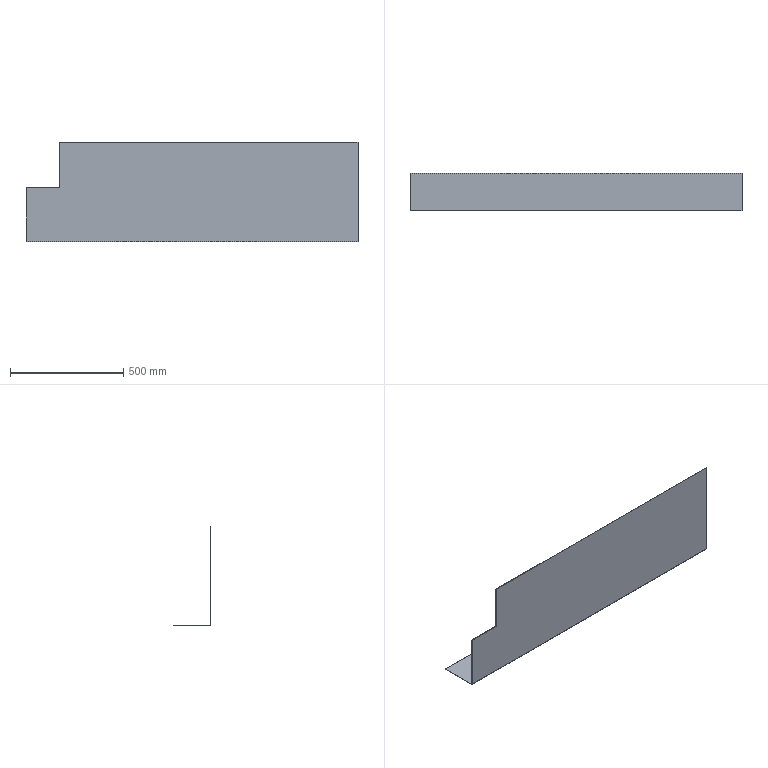Part | 1 solid | 16 faces | box 1465 x 167 x 440 mm | volume 1027988 mm3 | plane 14 | cylinder 2 | commonest cylinder face diameters 1.473 x1 3.873 x1
STEP:
#1=CARTESIAN_POINT('',(732.5,-81.563,0.));
#2=VERTEX_POINT('',#1);
#3=CARTESIAN_POINT('',(732.5,83.5,0.));
#4=VERTEX_POINT('',#3);
#5=CARTESIAN_POINT('',(732.5,83.5,0.));
#6=DIRECTION('',(0.,1.,0.));
#7=VECTOR('',#6,1000.);
#8=LINE('',#5,#7);
#9=EDGE_CURVE('',#2,#4,#8,.T.);
#10=ORIENTED_EDGE('',*,*,#9,.F.);
#11=CARTESIAN_POINT('',(732.5,-81.563,-1.2));
#12=VERTEX_POINT('',#11);
#13=CARTESIAN_POINT('',(732.5,-81.563,0.));
#14=DIRECTION('',(0.,0.,-1.));
#15=VECTOR('',#14,1000.);
#16=LINE('',#13,#15);
#17=EDGE_CURVE('',#2,#12,#16,.T.);
#18=ORIENTED_EDGE('',*,*,#17,.T.);
#19=CARTESIAN_POINT('',(732.5,83.5,-1.2));
#20=VERTEX_POINT('',#19);
#21=CARTESIAN_POINT('',(732.5,83.5,-1.2));
#22=DIRECTION('',(0.,1.,0.));
#23=VECTOR('',#22,1000.);
#24=LINE('',#21,#23);
#25=EDGE_CURVE('',#12,#20,#24,.T.);
#26=ORIENTED_EDGE('',*,*,#25,.T.);
#27=CARTESIAN_POINT('',(732.5,83.5,-1.2));
#28=DIRECTION('',(0.,0.,1.));
#29=VECTOR('',#28,1000.);
#30=LINE('',#27,#29);
#31=EDGE_CURVE('',#20,#4,#30,.T.);
#32=ORIENTED_EDGE('',*,*,#31,.T.);
#33=EDGE_LOOP('',(#10,#18,#26,#32));
#34=FACE_OUTER_BOUND('',#33,.T.);
#35=CARTESIAN_POINT('',(732.5,83.5,-1.2));
#36=DIRECTION('',(1.,0.,0.));
#37=DIRECTION('',(0.,1.,0.));
#38=AXIS2_PLACEMENT_3D('',#35,#36,#37);
#39=PLANE('',#38);
#40=ADVANCED_FACE('',(#34),#39,.T.);
#41=CARTESIAN_POINT('',(-732.5,-81.563,-1.2));
#42=VERTEX_POINT('',#41);
#43=CARTESIAN_POINT('',(732.5,-81.563,-1.2));
#44=DIRECTION('',(-1.,0.,0.));
#45=VECTOR('',#44,1000.);
#46=LINE('',#43,#45);
#47=EDGE_CURVE('',#12,#42,#46,.T.);
#48=ORIENTED_EDGE('',*,*,#47,.T.);
#49=CARTESIAN_POINT('',(-732.5,83.5,-1.2));
#50=VERTEX_POINT('',#49);
#51=CARTESIAN_POINT('',(-732.5,83.5,-1.2));
#52=DIRECTION('',(0.,-1.,0.));
#53=VECTOR('',#52,1000.);
#54=LINE('',#51,#53);
#55=EDGE_CURVE('',#50,#42,#54,.T.);
#56=ORIENTED_EDGE('',*,*,#55,.F.);
#57=CARTESIAN_POINT('',(-732.5,83.5,-1.2));
#58=DIRECTION('',(-1.,0.,0.));
#59=VECTOR('',#58,1000.);
#60=LINE('',#57,#59);
#61=EDGE_CURVE('',#20,#50,#60,.T.);
#62=ORIENTED_EDGE('',*,*,#61,.F.);
#63=ORIENTED_EDGE('',*,*,#25,.F.);
#64=EDGE_LOOP('',(#48,#56,#62,#63));
#65=FACE_OUTER_BOUND('',#64,.T.);
#66=CARTESIAN_POINT('',(0.,0.,-1.2));
#67=DIRECTION('',(0.,0.,1.));
#68=DIRECTION('',(1.,0.,0.));
#69=AXIS2_PLACEMENT_3D('',#66,#67,#68);
#70=PLANE('',#69);
#71=ADVANCED_FACE('',(#65),#70,.F.);
#72=CARTESIAN_POINT('',(-732.5,83.5,0.));
#73=VERTEX_POINT('',#72);
#74=CARTESIAN_POINT('',(-732.5,-81.563,0.));
#75=VERTEX_POINT('',#74);
#76=CARTESIAN_POINT('',(-732.5,83.5,0.));
#77=DIRECTION('',(0.,-1.,0.));
#78=VECTOR('',#77,1000.);
#79=LINE('',#76,#78);
#80=EDGE_CURVE('',#73,#75,#79,.T.);
#81=ORIENTED_EDGE('',*,*,#80,.T.);
#82=CARTESIAN_POINT('',(732.5,-81.563,0.));
#83=DIRECTION('',(-1.,0.,0.));
#84=VECTOR('',#83,1000.);
#85=LINE('',#82,#84);
#86=EDGE_CURVE('',#2,#75,#85,.T.);
#87=ORIENTED_EDGE('',*,*,#86,.F.);
#88=ORIENTED_EDGE('',*,*,#9,.T.);
#89=CARTESIAN_POINT('',(-732.5,83.5,0.));
#90=DIRECTION('',(-1.,0.,0.));
#91=VECTOR('',#90,1000.);
#92=LINE('',#89,#91);
#93=EDGE_CURVE('',#4,#73,#92,.T.);
#94=ORIENTED_EDGE('',*,*,#93,.T.);
#95=EDGE_LOOP('',(#81,#87,#88,#94));
#96=FACE_OUTER_BOUND('',#95,.T.);
#97=CARTESIAN_POINT('',(0.,0.,0.));
#98=DIRECTION('',(0.,0.,1.));
#99=DIRECTION('',(1.,0.,0.));
#100=AXIS2_PLACEMENT_3D('',#97,#98,#99);
#101=PLANE('',#100);
#102=ADVANCED_FACE('',(#96),#101,.T.);
#103=CARTESIAN_POINT('',(-732.5,-81.563,0.));
#104=DIRECTION('',(0.,0.,-1.));
#105=VECTOR('',#104,1000.);
#106=LINE('',#103,#105);
#107=EDGE_CURVE('',#75,#42,#106,.T.);
#108=ORIENTED_EDGE('',*,*,#107,.F.);
#109=ORIENTED_EDGE('',*,*,#80,.F.);
#110=CARTESIAN_POINT('',(-732.5,83.5,-1.2));
#111=DIRECTION('',(0.,0.,1.));
#112=VECTOR('',#111,1000.);
#113=LINE('',#110,#112);
#114=EDGE_CURVE('',#50,#73,#113,.T.);
#115=ORIENTED_EDGE('',*,*,#114,.F.);
#116=ORIENTED_EDGE('',*,*,#55,.T.);
#117=EDGE_LOOP('',(#108,#109,#115,#116));
#118=FACE_OUTER_BOUND('',#117,.T.);
#119=CARTESIAN_POINT('',(-732.5,83.5,-1.2));
#120=DIRECTION('',(-1.,0.,0.));
#121=DIRECTION('',(0.,0.,1.));
#122=AXIS2_PLACEMENT_3D('',#119,#120,#121);
#123=PLANE('',#122);
#124=ADVANCED_FACE('',(#118),#123,.T.);
#125=ORIENTED_EDGE('',*,*,#93,.F.);
#126=ORIENTED_EDGE('',*,*,#31,.F.);
#127=ORIENTED_EDGE('',*,*,#61,.T.);
#128=ORIENTED_EDGE('',*,*,#114,.T.);
#129=EDGE_LOOP('',(#125,#126,#127,#128));
#130=FACE_OUTER_BOUND('',#129,.T.);
#131=CARTESIAN_POINT('',(-732.5,83.5,-1.2));
#132=DIRECTION('',(0.,1.,0.));
#133=DIRECTION('',(0.,0.,1.));
#134=AXIS2_PLACEMENT_3D('',#131,#132,#133);
#135=PLANE('',#134);
#136=ADVANCED_FACE('',(#130),#135,.T.);
#137=CARTESIAN_POINT('',(-732.5,-82.3,0.7366));
#138=VERTEX_POINT('',#137);
#139=CARTESIAN_POINT('',(-732.5,-83.5,0.7366));
#140=VERTEX_POINT('',#139);
#141=CARTESIAN_POINT('',(-732.5,-83.5,0.7366));
#142=DIRECTION('',(0.,-1.,0.));
#143=VECTOR('',#142,1000.);
#144=LINE('',#141,#143);
#145=EDGE_CURVE('',#138,#140,#144,.T.);
#146=ORIENTED_EDGE('',*,*,#145,.F.);
#147=CARTESIAN_POINT('',(-732.5,-81.563,0.7366));
#148=DIRECTION('',(-1.,0.,0.));
#149=DIRECTION('',(0.,0.,-1.));
#150=AXIS2_PLACEMENT_3D('',#147,#148,#149);
#151=CIRCLE('',#150,0.7366);
#152=EDGE_CURVE('',#75,#138,#151,.T.);
#153=ORIENTED_EDGE('',*,*,#152,.F.);
#154=ORIENTED_EDGE('',*,*,#107,.T.);
#155=CARTESIAN_POINT('',(-732.5,-81.563,0.7366));
#156=DIRECTION('',(-1.,0.,0.));
#157=DIRECTION('',(0.,0.,-1.));
#158=AXIS2_PLACEMENT_3D('',#155,#156,#157);
#159=CIRCLE('',#158,1.937);
#160=EDGE_CURVE('',#42,#140,#159,.T.);
#161=ORIENTED_EDGE('',*,*,#160,.T.);
#162=EDGE_LOOP('',(#146,#153,#154,#161));
#163=FACE_OUTER_BOUND('',#162,.T.);
#164=CARTESIAN_POINT('',(-732.5,-81.563,0.7366));
#165=DIRECTION('',(-1.,0.,0.));
#166=DIRECTION('',(0.,0.,1.));
#167=AXIS2_PLACEMENT_3D('',#164,#165,#166);
#168=PLANE('',#167);
#169=ADVANCED_FACE('',(#163),#168,.T.);
#170=CARTESIAN_POINT('',(732.5,-82.3,0.7366));
#171=VERTEX_POINT('',#170);
#172=CARTESIAN_POINT('',(732.5,-81.563,0.7366));
#173=DIRECTION('',(1.,0.,0.));
#174=DIRECTION('',(0.,0.,-1.));
#175=AXIS2_PLACEMENT_3D('',#172,#173,#174);
#176=CIRCLE('',#175,0.7366);
#177=EDGE_CURVE('',#171,#2,#176,.T.);
#178=ORIENTED_EDGE('',*,*,#177,.F.);
#179=CARTESIAN_POINT('',(732.5,-83.5,0.7366));
#180=VERTEX_POINT('',#179);
#181=CARTESIAN_POINT('',(732.5,-82.3,0.7366));
#182=DIRECTION('',(0.,-1.,0.));
#183=VECTOR('',#182,1000.);
#184=LINE('',#181,#183);
#185=EDGE_CURVE('',#171,#180,#184,.T.);
#186=ORIENTED_EDGE('',*,*,#185,.T.);
#187=CARTESIAN_POINT('',(732.5,-81.563,0.7366));
#188=DIRECTION('',(1.,0.,0.));
#189=DIRECTION('',(0.,0.,-1.));
#190=AXIS2_PLACEMENT_3D('',#187,#188,#189);
#191=CIRCLE('',#190,1.937);
#192=EDGE_CURVE('',#180,#12,#191,.T.);
#193=ORIENTED_EDGE('',*,*,#192,.T.);
#194=ORIENTED_EDGE('',*,*,#17,.F.);
#195=EDGE_LOOP('',(#178,#186,#193,#194));
#196=FACE_OUTER_BOUND('',#195,.T.);
#197=CARTESIAN_POINT('',(732.5,-81.563,0.7366));
#198=DIRECTION('',(-1.,0.,0.));
#199=DIRECTION('',(0.,0.,1.));
#200=AXIS2_PLACEMENT_3D('',#197,#198,#199);
#201=PLANE('',#200);
#202=ADVANCED_FACE('',(#196),#201,.F.);
#203=ORIENTED_EDGE('',*,*,#47,.F.);
#204=ORIENTED_EDGE('',*,*,#192,.F.);
#205=CARTESIAN_POINT('',(0.,-83.5,0.7366));
#206=DIRECTION('',(1.,0.,0.));
#207=VECTOR('',#206,1000.);
#208=LINE('',#205,#207);
#209=EDGE_CURVE('',#140,#180,#208,.T.);
#210=ORIENTED_EDGE('',*,*,#209,.F.);
#211=ORIENTED_EDGE('',*,*,#160,.F.);
#212=EDGE_LOOP('',(#203,#204,#210,#211));
#213=FACE_OUTER_BOUND('',#212,.T.);
#214=CARTESIAN_POINT('',(732.5,-81.563,0.7366));
#215=DIRECTION('',(1.,0.,0.));
#216=DIRECTION('',(0.,-1.,0.));
#217=AXIS2_PLACEMENT_3D('',#214,#215,#216);
#218=CYLINDRICAL_SURFACE('',#217,1.937);
#219=ADVANCED_FACE('',(#213),#218,.T.);
#220=ORIENTED_EDGE('',*,*,#86,.T.);
#221=ORIENTED_EDGE('',*,*,#152,.T.);
#222=CARTESIAN_POINT('',(-732.5,-82.3,0.7366));
#223=DIRECTION('',(1.,0.,0.));
#224=VECTOR('',#223,1000.);
#225=LINE('',#222,#224);
#226=EDGE_CURVE('',#138,#171,#225,.T.);
#227=ORIENTED_EDGE('',*,*,#226,.T.);
#228=ORIENTED_EDGE('',*,*,#177,.T.);
#229=EDGE_LOOP('',(#220,#221,#227,#228));
#230=FACE_OUTER_BOUND('',#229,.T.);
#231=CARTESIAN_POINT('',(732.5,-81.563,0.7366));
#232=DIRECTION('',(1.,0.,0.));
#233=DIRECTION('',(0.,-1.,0.));
#234=AXIS2_PLACEMENT_3D('',#231,#232,#233);
#235=CYLINDRICAL_SURFACE('',#234,0.7366);
#236=ADVANCED_FACE('',(#230),#235,.F.);
#237=CARTESIAN_POINT('',(732.5,-83.5,438.8));
#238=VERTEX_POINT('',#237);
#239=CARTESIAN_POINT('',(732.5,-83.5,0.));
#240=DIRECTION('',(0.,0.,-1.));
#241=VECTOR('',#240,1000.);
#242=LINE('',#239,#241);
#243=EDGE_CURVE('',#238,#180,#242,.T.);
#244=ORIENTED_EDGE('',*,*,#243,.T.);
#245=ORIENTED_EDGE('',*,*,#185,.F.);
#246=CARTESIAN_POINT('',(732.5,-82.3,438.8));
#247=VERTEX_POINT('',#246);
#248=CARTESIAN_POINT('',(732.5,-82.3,0.));
#249=DIRECTION('',(0.,0.,-1.));
#250=VECTOR('',#249,1000.);
#251=LINE('',#248,#250);
#252=EDGE_CURVE('',#247,#171,#251,.T.);
#253=ORIENTED_EDGE('',*,*,#252,.F.);
#254=CARTESIAN_POINT('',(732.5,-83.5,438.8));
#255=DIRECTION('',(0.,1.,0.));
#256=VECTOR('',#255,1000.);
#257=LINE('',#254,#256);
#258=EDGE_CURVE('',#238,#247,#257,.T.);
#259=ORIENTED_EDGE('',*,*,#258,.F.);
#260=EDGE_LOOP('',(#244,#245,#253,#259));
#261=FACE_OUTER_BOUND('',#260,.T.);
#262=CARTESIAN_POINT('',(732.5,-83.5,0.));
#263=DIRECTION('',(1.,0.,0.));
#264=DIRECTION('',(0.,0.,-1.));
#265=AXIS2_PLACEMENT_3D('',#262,#263,#264);
#266=PLANE('',#265);
#267=ADVANCED_FACE('',(#261),#266,.T.);
#268=CARTESIAN_POINT('',(-732.5,-83.5,238.8));
#269=VERTEX_POINT('',#268);
#270=CARTESIAN_POINT('',(-732.5,-82.3,238.8));
#271=VERTEX_POINT('',#270);
#272=CARTESIAN_POINT('',(-732.5,-83.5,238.8));
#273=DIRECTION('',(0.,1.,0.));
#274=VECTOR('',#273,1000.);
#275=LINE('',#272,#274);
#276=EDGE_CURVE('',#269,#271,#275,.T.);
#277=ORIENTED_EDGE('',*,*,#276,.T.);
#278=CARTESIAN_POINT('',(-732.5,-82.3,0.));
#279=DIRECTION('',(0.,0.,1.));
#280=VECTOR('',#279,1000.);
#281=LINE('',#278,#280);
#282=EDGE_CURVE('',#138,#271,#281,.T.);
#283=ORIENTED_EDGE('',*,*,#282,.F.);
#284=ORIENTED_EDGE('',*,*,#145,.T.);
#285=CARTESIAN_POINT('',(-732.5,-83.5,438.8));
#286=DIRECTION('',(0.,0.,1.));
#287=VECTOR('',#286,1000.);
#288=LINE('',#285,#287);
#289=EDGE_CURVE('',#140,#269,#288,.T.);
#290=ORIENTED_EDGE('',*,*,#289,.T.);
#291=EDGE_LOOP('',(#277,#283,#284,#290));
#292=FACE_OUTER_BOUND('',#291,.T.);
#293=CARTESIAN_POINT('',(-732.5,-83.5,438.8));
#294=DIRECTION('',(-1.,0.,0.));
#295=DIRECTION('',(0.,0.,1.));
#296=AXIS2_PLACEMENT_3D('',#293,#294,#295);
#297=PLANE('',#296);
#298=ADVANCED_FACE('',(#292),#297,.T.);
#299=CARTESIAN_POINT('',(-582.5,-83.5,238.8));
#300=VERTEX_POINT('',#299);
#301=CARTESIAN_POINT('',(-732.5,-83.5,238.8));
#302=DIRECTION('',(-1.,0.,0.));
#303=VECTOR('',#302,1000.);
#304=LINE('',#301,#303);
#305=EDGE_CURVE('',#300,#269,#304,.T.);
#306=ORIENTED_EDGE('',*,*,#305,.T.);
#307=ORIENTED_EDGE('',*,*,#289,.F.);
#308=ORIENTED_EDGE('',*,*,#209,.T.);
#309=ORIENTED_EDGE('',*,*,#243,.F.);
#310=CARTESIAN_POINT('',(-582.5,-83.5,438.8));
#311=VERTEX_POINT('',#310);
#312=CARTESIAN_POINT('',(732.5,-83.5,438.8));
#313=DIRECTION('',(1.,0.,0.));
#314=VECTOR('',#313,1000.);
#315=LINE('',#312,#314);
#316=EDGE_CURVE('',#311,#238,#315,.T.);
#317=ORIENTED_EDGE('',*,*,#316,.F.);
#318=CARTESIAN_POINT('',(-582.5,-83.5,438.8));
#319=DIRECTION('',(0.,0.,-1.));
#320=VECTOR('',#319,1000.);
#321=LINE('',#318,#320);
#322=EDGE_CURVE('',#311,#300,#321,.T.);
#323=ORIENTED_EDGE('',*,*,#322,.T.);
#324=EDGE_LOOP('',(#306,#307,#308,#309,#317,#323));
#325=FACE_OUTER_BOUND('',#324,.T.);
#326=CARTESIAN_POINT('',(0.,-83.5,0.));
#327=DIRECTION('',(0.,-1.,0.));
#328=DIRECTION('',(0.,0.,-1.));
#329=AXIS2_PLACEMENT_3D('',#326,#327,#328);
#330=PLANE('',#329);
#331=ADVANCED_FACE('',(#325),#330,.T.);
#332=ORIENTED_EDGE('',*,*,#282,.T.);
#333=CARTESIAN_POINT('',(-582.5,-82.3,238.8));
#334=VERTEX_POINT('',#333);
#335=CARTESIAN_POINT('',(-732.5,-82.3,238.8));
#336=DIRECTION('',(-1.,0.,0.));
#337=VECTOR('',#336,1000.);
#338=LINE('',#335,#337);
#339=EDGE_CURVE('',#334,#271,#338,.T.);
#340=ORIENTED_EDGE('',*,*,#339,.F.);
#341=CARTESIAN_POINT('',(-582.5,-82.3,438.8));
#342=VERTEX_POINT('',#341);
#343=CARTESIAN_POINT('',(-582.5,-82.3,438.8));
#344=DIRECTION('',(0.,0.,-1.));
#345=VECTOR('',#344,1000.);
#346=LINE('',#343,#345);
#347=EDGE_CURVE('',#342,#334,#346,.T.);
#348=ORIENTED_EDGE('',*,*,#347,.F.);
#349=CARTESIAN_POINT('',(0.,-82.3,438.8));
#350=DIRECTION('',(1.,0.,0.));
#351=VECTOR('',#350,1000.);
#352=LINE('',#349,#351);
#353=EDGE_CURVE('',#342,#247,#352,.T.);
#354=ORIENTED_EDGE('',*,*,#353,.T.);
#355=ORIENTED_EDGE('',*,*,#252,.T.);
#356=ORIENTED_EDGE('',*,*,#226,.F.);
#357=EDGE_LOOP('',(#332,#340,#348,#354,#355,#356));
#358=FACE_OUTER_BOUND('',#357,.T.);
#359=CARTESIAN_POINT('',(0.,-82.3,0.));
#360=DIRECTION('',(0.,-1.,0.));
#361=DIRECTION('',(0.,0.,-1.));
#362=AXIS2_PLACEMENT_3D('',#359,#360,#361);
#363=PLANE('',#362);
#364=ADVANCED_FACE('',(#358),#363,.F.);
#365=CARTESIAN_POINT('',(-582.5,-83.5,438.8));
#366=DIRECTION('',(0.,1.,0.));
#367=VECTOR('',#366,1000.);
#368=LINE('',#365,#367);
#369=EDGE_CURVE('',#311,#342,#368,.T.);
#370=ORIENTED_EDGE('',*,*,#369,.F.);
#371=ORIENTED_EDGE('',*,*,#316,.T.);
#372=ORIENTED_EDGE('',*,*,#258,.T.);
#373=ORIENTED_EDGE('',*,*,#353,.F.);
#374=EDGE_LOOP('',(#370,#371,#372,#373));
#375=FACE_OUTER_BOUND('',#374,.T.);
#376=CARTESIAN_POINT('',(732.5,-83.5,438.8));
#377=DIRECTION('',(0.,0.,1.));
#378=DIRECTION('',(0.,-1.,0.));
#379=AXIS2_PLACEMENT_3D('',#376,#377,#378);
#380=PLANE('',#379);
#381=ADVANCED_FACE('',(#375),#380,.T.);
#382=ORIENTED_EDGE('',*,*,#339,.T.);
#383=ORIENTED_EDGE('',*,*,#276,.F.);
#384=ORIENTED_EDGE('',*,*,#305,.F.);
#385=CARTESIAN_POINT('',(-582.5,-83.5,238.8));
#386=DIRECTION('',(0.,1.,0.));
#387=VECTOR('',#386,1000.);
#388=LINE('',#385,#387);
#389=EDGE_CURVE('',#300,#334,#388,.T.);
#390=ORIENTED_EDGE('',*,*,#389,.T.);
#391=EDGE_LOOP('',(#382,#383,#384,#390));
#392=FACE_OUTER_BOUND('',#391,.T.);
#393=CARTESIAN_POINT('',(-732.5,-83.5,238.8));
#394=DIRECTION('',(0.,0.,-1.));
#395=DIRECTION('',(0.,1.,0.));
#396=AXIS2_PLACEMENT_3D('',#393,#394,#395);
#397=PLANE('',#396);
#398=ADVANCED_FACE('',(#392),#397,.F.);
#399=ORIENTED_EDGE('',*,*,#347,.T.);
#400=ORIENTED_EDGE('',*,*,#389,.F.);
#401=ORIENTED_EDGE('',*,*,#322,.F.);
#402=ORIENTED_EDGE('',*,*,#369,.T.);
#403=EDGE_LOOP('',(#399,#400,#401,#402));
#404=FACE_OUTER_BOUND('',#403,.T.);
#405=CARTESIAN_POINT('',(-582.5,-83.5,438.8));
#406=DIRECTION('',(1.,0.,0.));
#407=DIRECTION('',(0.,0.,-1.));
#408=AXIS2_PLACEMENT_3D('',#405,#406,#407);
#409=PLANE('',#408);
#410=ADVANCED_FACE('',(#404),#409,.F.);
#411=CLOSED_SHELL('',(#40,#71,#102,#124,#136,#169,#202,#219,#236,#267,#298,#331,#364,#381,#398,#410));
#412=MANIFOLD_SOLID_BREP('',#411);
#413=CARTESIAN_POINT('',(0.,0.,0.));
#414=DIRECTION('',(0.,0.,1.));
#415=DIRECTION('',(1.,0.,0.));
#416=AXIS2_PLACEMENT_3D('',#413,#414,#415);
#417=(LENGTH_UNIT()NAMED_UNIT(*)SI_UNIT(.MILLI.,.METRE.));
#418=UNCERTAINTY_MEASURE_WITH_UNIT(LENGTH_MEASURE(0.00001),#417,'','');
#419=(NAMED_UNIT(*)PLANE_ANGLE_UNIT()SI_UNIT($,.RADIAN.));
#420=(NAMED_UNIT(*)SI_UNIT($,.STERADIAN.)SOLID_ANGLE_UNIT());
#421=(GEOMETRIC_REPRESENTATION_CONTEXT(3)GLOBAL_UNCERTAINTY_ASSIGNED_CONTEXT((#418))GLOBAL_UNIT_ASSIGNED_CONTEXT((#417,#419,#420))REPRESENTATION_CONTEXT('',''));
#422=ADVANCED_BREP_SHAPE_REPRESENTATION('',(#412,#416),#421);